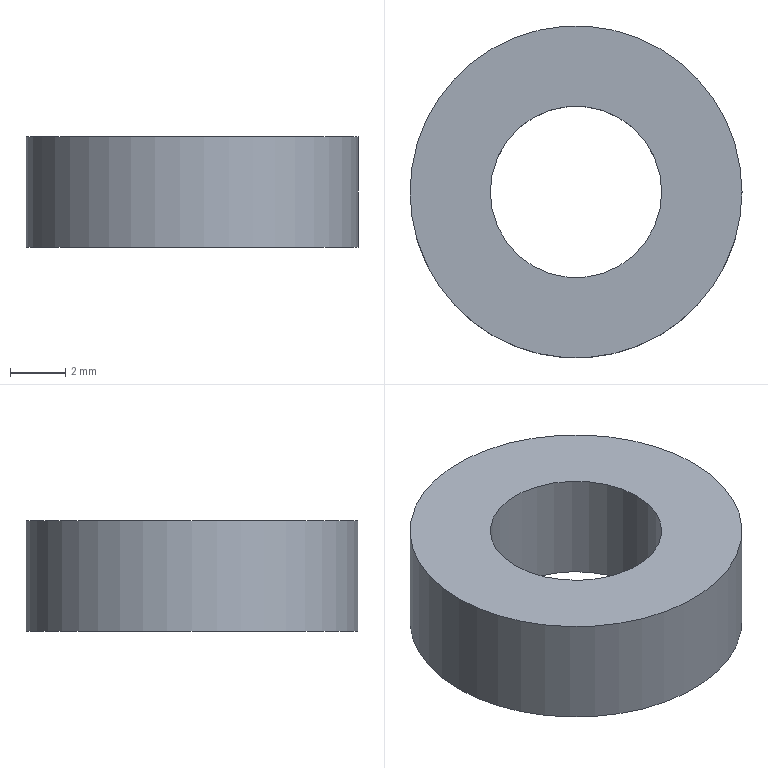Part | STEP file | 1 solid | 4 faces | box 12 x 12 x 4 mm | volume 331.627 mm3 | plane 2 | cylinder 2 | commonest cylinder face diameters 6.2 x1 12 x1
STEP:
#1=CARTESIAN_POINT('',(0.,0.,0.));
#2=DIRECTION('',(0.,0.,1.));
#3=DIRECTION('',(1.,0.,0.));
#4=AXIS2_PLACEMENT_3D('',#1,#2,#3);
#5=CARTESIAN_POINT('',(1387.633,370.98,-5.381));
#6=VERTEX_POINT('',#5);
#7=CARTESIAN_POINT('',(1390.733,370.98,-5.381));
#8=DIRECTION('',(0.,0.,1.));
#9=DIRECTION('',(-1.,0.,0.));
#10=AXIS2_PLACEMENT_3D('',#7,#8,#9);
#11=CIRCLE('',#10,3.1);
#12=CARTESIAN_POINT('',(1390.733,370.98,-5.381));
#13=DIRECTION('',(0.,0.,-1.));
#14=DIRECTION('',(-1.,0.,0.));
#15=AXIS2_PLACEMENT_3D('',#12,#13,#14);
#16=PLANE('',#15);
#17=CARTESIAN_POINT('',(3.1,0.));
#18=CARTESIAN_POINT('',(3.1,-5.369));
#19=CARTESIAN_POINT('',(-1.55,-2.685));
#20=CARTESIAN_POINT('',(-6.2,0.));
#21=CARTESIAN_POINT('',(-1.55,2.685));
#22=CARTESIAN_POINT('',(3.1,5.369));
#23=CARTESIAN_POINT('',(3.1,0.));
#24=(BOUNDED_CURVE()B_SPLINE_CURVE(2,(#17,#18,#19,#20,#21,#22,#23),.UNSPECIFIED.,.T.,.F.)B_SPLINE_CURVE_WITH_KNOTS((1,2,2,2,2,1),(-2.094,0.,2.094,4.189,6.283,8.378),.UNSPECIFIED.)CURVE()GEOMETRIC_REPRESENTATION_ITEM()RATIONAL_B_SPLINE_CURVE((1.,0.5,1.,0.5,1.,0.5,1.))REPRESENTATION_ITEM(''));
#25=(GEOMETRIC_REPRESENTATION_CONTEXT(2)PARAMETRIC_REPRESENTATION_CONTEXT()REPRESENTATION_CONTEXT('',''));
#26=DEFINITIONAL_REPRESENTATION('',(#24),#25);
#27=PCURVE('',#16,#26);
#28=CARTESIAN_POINT('',(1390.733,370.98,-5.381));
#29=DIRECTION('',(0.,0.,1.));
#30=DIRECTION('',(1.,0.,0.));
#31=AXIS2_PLACEMENT_3D('',#28,#29,#30);
#32=CYLINDRICAL_SURFACE('',#31,3.1);
#33=CARTESIAN_POINT('',(3.142,0.));
#34=DIRECTION('',(1.,0.));
#35=VECTOR('',#34,1.);
#36=LINE('',#33,#35);
#37=(GEOMETRIC_REPRESENTATION_CONTEXT(2)PARAMETRIC_REPRESENTATION_CONTEXT()REPRESENTATION_CONTEXT('',''));
#38=DEFINITIONAL_REPRESENTATION('',(#36),#37);
#39=PCURVE('',#32,#38);
#40=SURFACE_CURVE('',#11,(#27,#39),.PCURVE_S1.);
#41=EDGE_CURVE('',#6,#6,#40,.T.);
#42=ORIENTED_EDGE('',*,*,#41,.T.);
#43=EDGE_LOOP('',(#42));
#44=FACE_BOUND('',#43,.T.);
#45=CARTESIAN_POINT('',(1396.733,370.98,-5.381));
#46=VERTEX_POINT('',#45);
#47=CARTESIAN_POINT('',(1390.733,370.98,-5.381));
#48=DIRECTION('',(0.,0.,1.));
#49=DIRECTION('',(1.,0.,0.));
#50=AXIS2_PLACEMENT_3D('',#47,#48,#49);
#51=CIRCLE('',#50,6.);
#52=CARTESIAN_POINT('',(-6.,0.));
#53=CARTESIAN_POINT('',(-6.,10.392));
#54=CARTESIAN_POINT('',(3.,5.196));
#55=CARTESIAN_POINT('',(12.,0.));
#56=CARTESIAN_POINT('',(3.,-5.196));
#57=CARTESIAN_POINT('',(-6.,-10.392));
#58=CARTESIAN_POINT('',(-6.,0.));
#59=(BOUNDED_CURVE()B_SPLINE_CURVE(2,(#52,#53,#54,#55,#56,#57,#58),.UNSPECIFIED.,.T.,.F.)B_SPLINE_CURVE_WITH_KNOTS((1,2,2,2,2,1),(-2.094,0.,2.094,4.189,6.283,8.378),.UNSPECIFIED.)CURVE()GEOMETRIC_REPRESENTATION_ITEM()RATIONAL_B_SPLINE_CURVE((1.,0.5,1.,0.5,1.,0.5,1.))REPRESENTATION_ITEM(''));
#60=(GEOMETRIC_REPRESENTATION_CONTEXT(2)PARAMETRIC_REPRESENTATION_CONTEXT()REPRESENTATION_CONTEXT('',''));
#61=DEFINITIONAL_REPRESENTATION('',(#59),#60);
#62=PCURVE('',#16,#61);
#63=CARTESIAN_POINT('',(1390.733,370.98,-1.381));
#64=DIRECTION('',(0.,0.,-1.));
#65=DIRECTION('',(-1.,0.,0.));
#66=AXIS2_PLACEMENT_3D('',#63,#64,#65);
#67=CYLINDRICAL_SURFACE('',#66,6.);
#68=CARTESIAN_POINT('',(9.425,4.));
#69=DIRECTION('',(-1.,0.));
#70=VECTOR('',#69,1.);
#71=LINE('',#68,#70);
#72=(GEOMETRIC_REPRESENTATION_CONTEXT(2)PARAMETRIC_REPRESENTATION_CONTEXT()REPRESENTATION_CONTEXT('',''));
#73=DEFINITIONAL_REPRESENTATION('',(#71),#72);
#74=PCURVE('',#67,#73);
#75=SURFACE_CURVE('',#51,(#62,#74),.PCURVE_S1.);
#76=EDGE_CURVE('',#46,#46,#75,.T.);
#77=ORIENTED_EDGE('',*,*,#76,.F.);
#78=EDGE_LOOP('',(#77));
#79=FACE_BOUND('',#78,.T.);
#80=ADVANCED_FACE('',(#44,#79),#16,.T.);
#81=CARTESIAN_POINT('',(1387.633,370.98,-1.381));
#82=VERTEX_POINT('',#81);
#83=CARTESIAN_POINT('',(1390.733,370.98,-1.381));
#84=DIRECTION('',(0.,0.,1.));
#85=DIRECTION('',(-1.,0.,0.));
#86=AXIS2_PLACEMENT_3D('',#83,#84,#85);
#87=CIRCLE('',#86,3.1);
#88=CARTESIAN_POINT('',(1390.733,370.98,-1.381));
#89=DIRECTION('',(0.,0.,1.));
#90=DIRECTION('',(1.,0.,0.));
#91=AXIS2_PLACEMENT_3D('',#88,#89,#90);
#92=PLANE('',#91);
#93=CARTESIAN_POINT('',(0.,0.));
#94=DIRECTION('',(-1.,0.));
#95=AXIS2_PLACEMENT_2D('',#93,#94);
#96=CIRCLE('',#95,3.1);
#97=(GEOMETRIC_REPRESENTATION_CONTEXT(2)PARAMETRIC_REPRESENTATION_CONTEXT()REPRESENTATION_CONTEXT('',''));
#98=DEFINITIONAL_REPRESENTATION('',(#96),#97);
#99=PCURVE('',#92,#98);
#100=CARTESIAN_POINT('',(3.142,4.));
#101=DIRECTION('',(1.,0.));
#102=VECTOR('',#101,1.);
#103=LINE('',#100,#102);
#104=(GEOMETRIC_REPRESENTATION_CONTEXT(2)PARAMETRIC_REPRESENTATION_CONTEXT()REPRESENTATION_CONTEXT('',''));
#105=DEFINITIONAL_REPRESENTATION('',(#103),#104);
#106=PCURVE('',#32,#105);
#107=SURFACE_CURVE('',#87,(#99,#106),.PCURVE_S1.);
#108=EDGE_CURVE('',#82,#82,#107,.T.);
#109=ORIENTED_EDGE('',*,*,#108,.F.);
#110=EDGE_LOOP('',(#109));
#111=FACE_BOUND('',#110,.T.);
#112=CARTESIAN_POINT('',(1396.733,370.98,-1.381));
#113=VERTEX_POINT('',#112);
#114=CARTESIAN_POINT('',(1390.733,370.98,-1.381));
#115=DIRECTION('',(0.,0.,-1.));
#116=DIRECTION('',(1.,0.,0.));
#117=AXIS2_PLACEMENT_3D('',#114,#115,#116);
#118=CIRCLE('',#117,6.);
#119=CARTESIAN_POINT('',(6.,0.));
#120=CARTESIAN_POINT('',(6.,-10.392));
#121=CARTESIAN_POINT('',(-3.,-5.196));
#122=CARTESIAN_POINT('',(-12.,0.));
#123=CARTESIAN_POINT('',(-3.,5.196));
#124=CARTESIAN_POINT('',(6.,10.392));
#125=CARTESIAN_POINT('',(6.,0.));
#126=(BOUNDED_CURVE()B_SPLINE_CURVE(2,(#119,#120,#121,#122,#123,#124,#125),.UNSPECIFIED.,.T.,.F.)B_SPLINE_CURVE_WITH_KNOTS((1,2,2,2,2,1),(-2.094,0.,2.094,4.189,6.283,8.378),.UNSPECIFIED.)CURVE()GEOMETRIC_REPRESENTATION_ITEM()RATIONAL_B_SPLINE_CURVE((1.,0.5,1.,0.5,1.,0.5,1.))REPRESENTATION_ITEM(''));
#127=(GEOMETRIC_REPRESENTATION_CONTEXT(2)PARAMETRIC_REPRESENTATION_CONTEXT()REPRESENTATION_CONTEXT('',''));
#128=DEFINITIONAL_REPRESENTATION('',(#126),#127);
#129=PCURVE('',#92,#128);
#130=CARTESIAN_POINT('',(3.142,0.));
#131=DIRECTION('',(1.,0.));
#132=VECTOR('',#131,1.);
#133=LINE('',#130,#132);
#134=(GEOMETRIC_REPRESENTATION_CONTEXT(2)PARAMETRIC_REPRESENTATION_CONTEXT()REPRESENTATION_CONTEXT('',''));
#135=DEFINITIONAL_REPRESENTATION('',(#133),#134);
#136=PCURVE('',#67,#135);
#137=SURFACE_CURVE('',#118,(#129,#136),.PCURVE_S1.);
#138=EDGE_CURVE('',#113,#113,#137,.T.);
#139=ORIENTED_EDGE('',*,*,#138,.F.);
#140=EDGE_LOOP('',(#139));
#141=FACE_BOUND('',#140,.T.);
#142=ADVANCED_FACE('',(#111,#141),#92,.T.);
#143=ORIENTED_EDGE('',*,*,#76,.T.);
#144=CARTESIAN_POINT('',(1396.733,370.98,-1.381));
#145=CARTESIAN_POINT('',(1396.733,370.98,-5.381));
#146=B_SPLINE_CURVE_WITH_KNOTS('',1,(#144,#145),.UNSPECIFIED.,.F.,.F.,(2,2),(0.,4.),.PIECEWISE_BEZIER_KNOTS.);
#147=CARTESIAN_POINT('',(3.142,0.));
#148=DIRECTION('',(0.,1.));
#149=VECTOR('',#148,1.);
#150=LINE('',#147,#149);
#151=(GEOMETRIC_REPRESENTATION_CONTEXT(2)PARAMETRIC_REPRESENTATION_CONTEXT()REPRESENTATION_CONTEXT('',''));
#152=DEFINITIONAL_REPRESENTATION('',(#150),#151);
#153=PCURVE('',#67,#152);
#154=CARTESIAN_POINT('',(9.425,0.));
#155=DIRECTION('',(0.,1.));
#156=VECTOR('',#155,1.);
#157=LINE('',#154,#156);
#158=(GEOMETRIC_REPRESENTATION_CONTEXT(2)PARAMETRIC_REPRESENTATION_CONTEXT()REPRESENTATION_CONTEXT('',''));
#159=DEFINITIONAL_REPRESENTATION('',(#157),#158);
#160=PCURVE('',#67,#159);
#161=SEAM_CURVE('',#146,(#153,#160),.PCURVE_S1.);
#162=EDGE_CURVE('',#113,#46,#161,.T.);
#163=ORIENTED_EDGE('',*,*,#162,.F.);
#164=ORIENTED_EDGE('',*,*,#138,.T.);
#165=ORIENTED_EDGE('',*,*,#162,.T.);
#166=EDGE_LOOP('',(#143,#163,#164,#165));
#167=FACE_BOUND('',#166,.T.);
#168=ADVANCED_FACE('',(#167),#67,.T.);
#169=ORIENTED_EDGE('',*,*,#108,.F.);
#170=CARTESIAN_POINT('',(1387.633,370.98,-5.381));
#171=CARTESIAN_POINT('',(1387.633,370.98,-1.381));
#172=B_SPLINE_CURVE_WITH_KNOTS('',1,(#170,#171),.UNSPECIFIED.,.F.,.F.,(2,2),(0.,4.),.PIECEWISE_BEZIER_KNOTS.);
#173=CARTESIAN_POINT('',(3.142,0.));
#174=DIRECTION('',(0.,1.));
#175=VECTOR('',#174,1.);
#176=LINE('',#173,#175);
#177=(GEOMETRIC_REPRESENTATION_CONTEXT(2)PARAMETRIC_REPRESENTATION_CONTEXT()REPRESENTATION_CONTEXT('',''));
#178=DEFINITIONAL_REPRESENTATION('',(#176),#177);
#179=PCURVE('',#32,#178);
#180=CARTESIAN_POINT('',(9.425,0.));
#181=DIRECTION('',(0.,1.));
#182=VECTOR('',#181,1.);
#183=LINE('',#180,#182);
#184=(GEOMETRIC_REPRESENTATION_CONTEXT(2)PARAMETRIC_REPRESENTATION_CONTEXT()REPRESENTATION_CONTEXT('',''));
#185=DEFINITIONAL_REPRESENTATION('',(#183),#184);
#186=PCURVE('',#32,#185);
#187=SEAM_CURVE('',#172,(#179,#186),.PCURVE_S1.);
#188=EDGE_CURVE('',#6,#82,#187,.T.);
#189=ORIENTED_EDGE('',*,*,#188,.F.);
#190=ORIENTED_EDGE('',*,*,#41,.T.);
#191=ORIENTED_EDGE('',*,*,#188,.T.);
#192=EDGE_LOOP('',(#169,#189,#190,#191));
#193=FACE_BOUND('',#192,.F.);
#194=ADVANCED_FACE('',(#193),#32,.F.);
#195=CLOSED_SHELL('',(#80,#142,#168,#194));
#196=MANIFOLD_SOLID_BREP('',#195);
#197=(LENGTH_UNIT()NAMED_UNIT(*)SI_UNIT(.MILLI.,.METRE.));
#198=UNCERTAINTY_MEASURE_WITH_UNIT(LENGTH_MEASURE(0.00001),#197,'','');
#199=(NAMED_UNIT(*)PLANE_ANGLE_UNIT()SI_UNIT($,.RADIAN.));
#200=(NAMED_UNIT(*)SI_UNIT($,.STERADIAN.)SOLID_ANGLE_UNIT());
#201=(GEOMETRIC_REPRESENTATION_CONTEXT(3)GLOBAL_UNCERTAINTY_ASSIGNED_CONTEXT((#198))GLOBAL_UNIT_ASSIGNED_CONTEXT((#197,#199,#200))REPRESENTATION_CONTEXT('',''));
#202=ADVANCED_BREP_SHAPE_REPRESENTATION('',(#4,#196),#201);